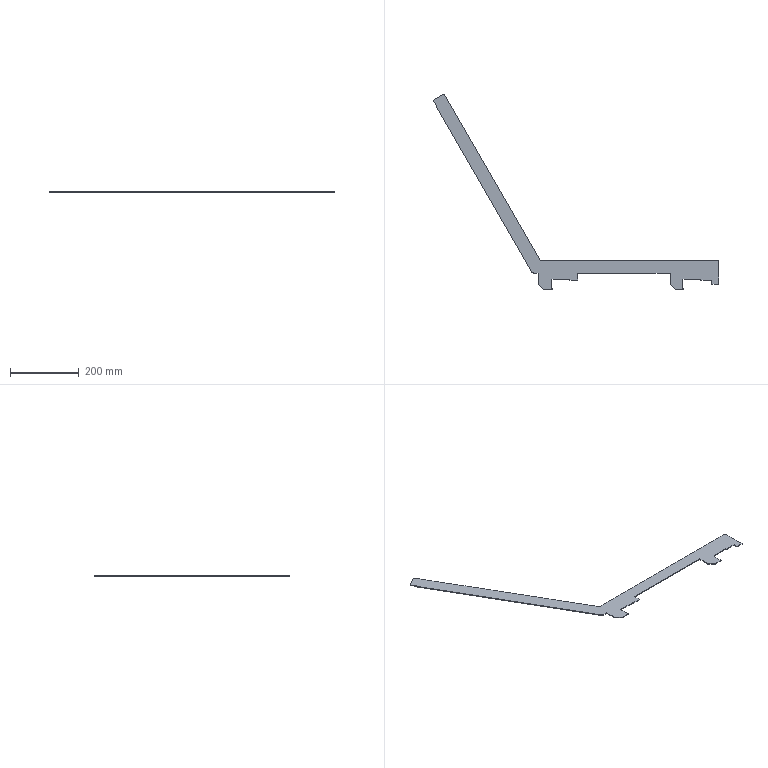Part | STEP file | zh001-1 | 1 solid | 35 faces | box 827.736 x 568.01 x 2 mm | volume 95326 mm3 | plane 32 | cylinder 3 | commonest cylinder face diameters 4 x2 20 x1
STEP:
#1=CARTESIAN_POINT('',(-259.956,-10.5,0.));
#2=VERTEX_POINT('',#1);
#3=CARTESIAN_POINT('',(-268.617,-5.5,0.));
#4=VERTEX_POINT('',#3);
#5=CARTESIAN_POINT('',(-259.956,-0.5,0.));
#6=DIRECTION('',(0.,0.,-1.));
#7=DIRECTION('',(1.,0.,0.));
#8=AXIS2_PLACEMENT_3D('',#5,#6,#7);
#9=CIRCLE('',#8,10.);
#10=EDGE_CURVE('',#2,#4,#9,.T.);
#11=ORIENTED_EDGE('',*,*,#10,.F.);
#12=CARTESIAN_POINT('',(-248.981,-10.5,0.));
#13=VERTEX_POINT('',#12);
#14=CARTESIAN_POINT('',(0.,-10.5,0.));
#15=DIRECTION('',(-1.,0.,0.));
#16=VECTOR('',#15,1000.);
#17=LINE('',#14,#16);
#18=EDGE_CURVE('',#13,#2,#17,.T.);
#19=ORIENTED_EDGE('',*,*,#18,.F.);
#20=CARTESIAN_POINT('',(-248.981,-43.,0.));
#21=VERTEX_POINT('',#20);
#22=CARTESIAN_POINT('',(-248.981,0.,0.));
#23=DIRECTION('',(0.,1.,0.));
#24=VECTOR('',#23,1000.);
#25=LINE('',#22,#24);
#26=EDGE_CURVE('',#21,#13,#25,.T.);
#27=ORIENTED_EDGE('',*,*,#26,.F.);
#28=CARTESIAN_POINT('',(-232.981,-59.,0.));
#29=VERTEX_POINT('',#28);
#30=CARTESIAN_POINT('',(-232.981,-59.,0.));
#31=DIRECTION('',(-0.7071,0.7071,0.));
#32=VECTOR('',#31,1000.);
#33=LINE('',#30,#32);
#34=EDGE_CURVE('',#29,#21,#33,.T.);
#35=ORIENTED_EDGE('',*,*,#34,.F.);
#36=CARTESIAN_POINT('',(-206.481,-59.,0.));
#37=VERTEX_POINT('',#36);
#38=CARTESIAN_POINT('',(0.,-59.,0.));
#39=DIRECTION('',(-1.,0.,0.));
#40=VECTOR('',#39,1000.);
#41=LINE('',#38,#40);
#42=EDGE_CURVE('',#37,#29,#41,.T.);
#43=ORIENTED_EDGE('',*,*,#42,.F.);
#44=CARTESIAN_POINT('',(-206.481,-56.,0.));
#45=VERTEX_POINT('',#44);
#46=CARTESIAN_POINT('',(-206.481,0.,0.));
#47=DIRECTION('',(0.,-1.,0.));
#48=VECTOR('',#47,1000.);
#49=LINE('',#46,#48);
#50=EDGE_CURVE('',#45,#37,#49,.T.);
#51=ORIENTED_EDGE('',*,*,#50,.F.);
#52=CARTESIAN_POINT('',(-208.981,-56.,0.));
#53=VERTEX_POINT('',#52);
#54=CARTESIAN_POINT('',(0.,-56.,0.));
#55=DIRECTION('',(1.,0.,0.));
#56=VECTOR('',#55,1000.);
#57=LINE('',#54,#56);
#58=EDGE_CURVE('',#53,#45,#57,.T.);
#59=ORIENTED_EDGE('',*,*,#58,.F.);
#60=CARTESIAN_POINT('',(-208.981,-28.,0.));
#61=VERTEX_POINT('',#60);
#62=CARTESIAN_POINT('',(-208.981,0.,0.));
#63=DIRECTION('',(0.,-1.,0.));
#64=VECTOR('',#63,1000.);
#65=LINE('',#62,#64);
#66=EDGE_CURVE('',#61,#53,#65,.T.);
#67=ORIENTED_EDGE('',*,*,#66,.F.);
#68=CARTESIAN_POINT('',(-156.981,-28.,0.));
#69=VERTEX_POINT('',#68);
#70=CARTESIAN_POINT('',(0.,-28.,0.));
#71=DIRECTION('',(-1.,0.,0.));
#72=VECTOR('',#71,1000.);
#73=LINE('',#70,#72);
#74=EDGE_CURVE('',#69,#61,#73,.T.);
#75=ORIENTED_EDGE('',*,*,#74,.F.);
#76=CARTESIAN_POINT('',(-156.981,-30.5,0.));
#77=VERTEX_POINT('',#76);
#78=CARTESIAN_POINT('',(-156.981,0.,0.));
#79=DIRECTION('',(0.,1.,0.));
#80=VECTOR('',#79,1000.);
#81=LINE('',#78,#80);
#82=EDGE_CURVE('',#77,#69,#81,.T.);
#83=ORIENTED_EDGE('',*,*,#82,.F.);
#84=CARTESIAN_POINT('',(-134.519,-30.5,0.));
#85=VERTEX_POINT('',#84);
#86=CARTESIAN_POINT('',(0.,-30.5,0.));
#87=DIRECTION('',(-1.,0.,0.));
#88=VECTOR('',#87,1000.);
#89=LINE('',#86,#88);
#90=EDGE_CURVE('',#85,#77,#89,.T.);
#91=ORIENTED_EDGE('',*,*,#90,.F.);
#92=CARTESIAN_POINT('',(-134.519,-10.5,0.));
#93=VERTEX_POINT('',#92);
#94=CARTESIAN_POINT('',(-134.519,0.,0.));
#95=DIRECTION('',(0.,-1.,0.));
#96=VECTOR('',#95,1000.);
#97=LINE('',#94,#96);
#98=EDGE_CURVE('',#93,#85,#97,.T.);
#99=ORIENTED_EDGE('',*,*,#98,.F.);
#100=CARTESIAN_POINT('',(133.519,-10.5,0.));
#101=VERTEX_POINT('',#100);
#102=CARTESIAN_POINT('',(0.,-10.5,0.));
#103=DIRECTION('',(-1.,0.,0.));
#104=VECTOR('',#103,1000.);
#105=LINE('',#102,#104);
#106=EDGE_CURVE('',#101,#93,#105,.T.);
#107=ORIENTED_EDGE('',*,*,#106,.F.);
#108=CARTESIAN_POINT('',(133.519,-43.,0.));
#109=VERTEX_POINT('',#108);
#110=CARTESIAN_POINT('',(133.519,0.,0.));
#111=DIRECTION('',(0.,1.,0.));
#112=VECTOR('',#111,1000.);
#113=LINE('',#110,#112);
#114=EDGE_CURVE('',#109,#101,#113,.T.);
#115=ORIENTED_EDGE('',*,*,#114,.F.);
#116=CARTESIAN_POINT('',(149.519,-59.,0.));
#117=VERTEX_POINT('',#116);
#118=CARTESIAN_POINT('',(149.519,-59.,0.));
#119=DIRECTION('',(-0.7071,0.7071,0.));
#120=VECTOR('',#119,1000.);
#121=LINE('',#118,#120);
#122=EDGE_CURVE('',#117,#109,#121,.T.);
#123=ORIENTED_EDGE('',*,*,#122,.F.);
#124=CARTESIAN_POINT('',(173.519,-59.,0.));
#125=VERTEX_POINT('',#124);
#126=CARTESIAN_POINT('',(0.,-59.,0.));
#127=DIRECTION('',(-1.,0.,0.));
#128=VECTOR('',#127,1000.);
#129=LINE('',#126,#128);
#130=EDGE_CURVE('',#125,#117,#129,.T.);
#131=ORIENTED_EDGE('',*,*,#130,.F.);
#132=CARTESIAN_POINT('',(173.519,-56.,0.));
#133=VERTEX_POINT('',#132);
#134=CARTESIAN_POINT('',(173.519,0.,0.));
#135=DIRECTION('',(0.,-1.,0.));
#136=VECTOR('',#135,1000.);
#137=LINE('',#134,#136);
#138=EDGE_CURVE('',#133,#125,#137,.T.);
#139=ORIENTED_EDGE('',*,*,#138,.F.);
#140=CARTESIAN_POINT('',(171.019,-56.,0.));
#141=VERTEX_POINT('',#140);
#142=CARTESIAN_POINT('',(0.,-56.,0.));
#143=DIRECTION('',(1.,0.,0.));
#144=VECTOR('',#143,1000.);
#145=LINE('',#142,#144);
#146=EDGE_CURVE('',#141,#133,#145,.T.);
#147=ORIENTED_EDGE('',*,*,#146,.F.);
#148=CARTESIAN_POINT('',(171.019,-28.,0.));
#149=VERTEX_POINT('',#148);
#150=CARTESIAN_POINT('',(171.019,0.,0.));
#151=DIRECTION('',(0.,-1.,0.));
#152=VECTOR('',#151,1000.);
#153=LINE('',#150,#152);
#154=EDGE_CURVE('',#149,#141,#153,.T.);
#155=ORIENTED_EDGE('',*,*,#154,.F.);
#156=CARTESIAN_POINT('',(223.019,-28.,0.));
#157=VERTEX_POINT('',#156);
#158=CARTESIAN_POINT('',(0.,-28.,0.));
#159=DIRECTION('',(-1.,0.,0.));
#160=VECTOR('',#159,1000.);
#161=LINE('',#158,#160);
#162=EDGE_CURVE('',#157,#149,#161,.T.);
#163=ORIENTED_EDGE('',*,*,#162,.F.);
#164=CARTESIAN_POINT('',(223.019,-30.5,0.));
#165=VERTEX_POINT('',#164);
#166=CARTESIAN_POINT('',(223.019,0.,0.));
#167=DIRECTION('',(0.,1.,0.));
#168=VECTOR('',#167,1000.);
#169=LINE('',#166,#168);
#170=EDGE_CURVE('',#165,#157,#169,.T.);
#171=ORIENTED_EDGE('',*,*,#170,.F.);
#172=CARTESIAN_POINT('',(254.235,-30.5,0.));
#173=VERTEX_POINT('',#172);
#174=CARTESIAN_POINT('',(0.,-30.5,0.));
#175=DIRECTION('',(-1.,0.,0.));
#176=VECTOR('',#175,1000.);
#177=LINE('',#174,#176);
#178=EDGE_CURVE('',#173,#165,#177,.T.);
#179=ORIENTED_EDGE('',*,*,#178,.F.);
#180=CARTESIAN_POINT('',(254.235,-42.5,0.));
#181=VERTEX_POINT('',#180);
#182=CARTESIAN_POINT('',(254.235,0.,0.));
#183=DIRECTION('',(0.,1.,0.));
#184=VECTOR('',#183,1000.);
#185=LINE('',#182,#184);
#186=EDGE_CURVE('',#181,#173,#185,.T.);
#187=ORIENTED_EDGE('',*,*,#186,.F.);
#188=CARTESIAN_POINT('',(274.519,-42.5,0.));
#189=VERTEX_POINT('',#188);
#190=CARTESIAN_POINT('',(0.,-42.5,0.));
#191=DIRECTION('',(-1.,0.,0.));
#192=VECTOR('',#191,1000.);
#193=LINE('',#190,#192);
#194=EDGE_CURVE('',#189,#181,#193,.T.);
#195=ORIENTED_EDGE('',*,*,#194,.F.);
#196=CARTESIAN_POINT('',(274.519,23.5,0.));
#197=VERTEX_POINT('',#196);
#198=CARTESIAN_POINT('',(274.519,0.,0.));
#199=DIRECTION('',(0.,-1.,0.));
#200=VECTOR('',#199,1000.);
#201=LINE('',#198,#200);
#202=EDGE_CURVE('',#197,#189,#201,.T.);
#203=ORIENTED_EDGE('',*,*,#202,.F.);
#204=CARTESIAN_POINT('',(272.519,25.5,0.));
#205=VERTEX_POINT('',#204);
#206=CARTESIAN_POINT('',(272.519,23.5,0.));
#207=DIRECTION('',(0.,0.,-1.));
#208=DIRECTION('',(1.,0.,0.));
#209=AXIS2_PLACEMENT_3D('',#206,#207,#208);
#210=CIRCLE('',#209,2.);
#211=EDGE_CURVE('',#205,#197,#210,.T.);
#212=ORIENTED_EDGE('',*,*,#211,.F.);
#213=CARTESIAN_POINT('',(-242.636,25.5,0.));
#214=VERTEX_POINT('',#213);
#215=CARTESIAN_POINT('',(0.,25.5,0.));
#216=DIRECTION('',(1.,0.,0.));
#217=VECTOR('',#216,1000.);
#218=LINE('',#215,#217);
#219=EDGE_CURVE('',#214,#205,#218,.T.);
#220=ORIENTED_EDGE('',*,*,#219,.F.);
#221=CARTESIAN_POINT('',(-521.213,508.01,0.));
#222=VERTEX_POINT('',#221);
#223=CARTESIAN_POINT('',(-521.213,508.01,0.));
#224=DIRECTION('',(0.5,-0.866,0.));
#225=VECTOR('',#224,1000.);
#226=LINE('',#223,#225);
#227=EDGE_CURVE('',#222,#214,#226,.T.);
#228=ORIENTED_EDGE('',*,*,#227,.F.);
#229=CARTESIAN_POINT('',(-523.945,508.742,0.));
#230=VERTEX_POINT('',#229);
#231=CARTESIAN_POINT('',(-522.945,507.01,0.));
#232=DIRECTION('',(0.,0.,-1.));
#233=DIRECTION('',(1.,0.,0.));
#234=AXIS2_PLACEMENT_3D('',#231,#232,#233);
#235=CIRCLE('',#234,2.);
#236=EDGE_CURVE('',#230,#222,#235,.T.);
#237=ORIENTED_EDGE('',*,*,#236,.F.);
#238=CARTESIAN_POINT('',(-553.217,491.842,0.));
#239=VERTEX_POINT('',#238);
#240=CARTESIAN_POINT('',(-553.217,491.842,0.));
#241=DIRECTION('',(0.866,0.5,0.));
#242=VECTOR('',#241,1000.);
#243=LINE('',#240,#242);
#244=EDGE_CURVE('',#239,#230,#243,.T.);
#245=ORIENTED_EDGE('',*,*,#244,.F.);
#246=CARTESIAN_POINT('',(-543.117,474.348,0.));
#247=VERTEX_POINT('',#246);
#248=CARTESIAN_POINT('',(-543.117,474.348,0.));
#249=DIRECTION('',(-0.5,0.866,0.));
#250=VECTOR('',#249,1000.);
#251=LINE('',#248,#250);
#252=EDGE_CURVE('',#247,#239,#251,.T.);
#253=ORIENTED_EDGE('',*,*,#252,.F.);
#254=CARTESIAN_POINT('',(-545.022,473.248,0.));
#255=VERTEX_POINT('',#254);
#256=CARTESIAN_POINT('',(-545.022,473.248,0.));
#257=DIRECTION('',(0.866,0.5,0.));
#258=VECTOR('',#257,1000.);
#259=LINE('',#256,#258);
#260=EDGE_CURVE('',#255,#247,#259,.T.);
#261=ORIENTED_EDGE('',*,*,#260,.F.);
#262=CARTESIAN_POINT('',(-268.617,-5.5,0.));
#263=DIRECTION('',(-0.5,0.866,0.));
#264=VECTOR('',#263,1000.);
#265=LINE('',#262,#264);
#266=EDGE_CURVE('',#4,#255,#265,.T.);
#267=ORIENTED_EDGE('',*,*,#266,.F.);
#268=EDGE_LOOP('',(#11,#19,#27,#35,#43,#51,#59,#67,#75,#83,#91,#99,#107,#115,#123,#131,#139,#147,#155,#163,#171,#179,#187,#195,#203,#212,#220,#228,#237,#245,#253,#261,#267));
#269=FACE_OUTER_BOUND('',#268,.T.);
#270=CARTESIAN_POINT('',(0.,0.,0.));
#271=DIRECTION('',(0.,0.,-1.));
#272=DIRECTION('',(-1.,0.,0.));
#273=AXIS2_PLACEMENT_3D('',#270,#271,#272);
#274=PLANE('',#273);
#275=ADVANCED_FACE('',(#269),#274,.F.);
#276=ORIENTED_EDGE('',*,*,#266,.T.);
#277=CARTESIAN_POINT('',(-545.022,473.248,-2.));
#278=VERTEX_POINT('',#277);
#279=CARTESIAN_POINT('',(-545.022,473.248,-2.));
#280=DIRECTION('',(0.,0.,-1.));
#281=VECTOR('',#280,1000.);
#282=LINE('',#279,#281);
#283=EDGE_CURVE('',#255,#278,#282,.T.);
#284=ORIENTED_EDGE('',*,*,#283,.T.);
#285=CARTESIAN_POINT('',(-268.617,-5.5,-2.));
#286=VERTEX_POINT('',#285);
#287=CARTESIAN_POINT('',(-545.022,473.248,-2.));
#288=DIRECTION('',(0.5,-0.866,0.));
#289=VECTOR('',#288,1000.);
#290=LINE('',#287,#289);
#291=EDGE_CURVE('',#278,#286,#290,.T.);
#292=ORIENTED_EDGE('',*,*,#291,.T.);
#293=CARTESIAN_POINT('',(-268.617,-5.5,-2.));
#294=DIRECTION('',(0.,0.,1.));
#295=VECTOR('',#294,1000.);
#296=LINE('',#293,#295);
#297=EDGE_CURVE('',#286,#4,#296,.T.);
#298=ORIENTED_EDGE('',*,*,#297,.T.);
#299=EDGE_LOOP('',(#276,#284,#292,#298));
#300=FACE_OUTER_BOUND('',#299,.T.);
#301=CARTESIAN_POINT('',(-545.022,473.248,-2.));
#302=DIRECTION('',(-0.866,-0.5,0.));
#303=DIRECTION('',(0.5,-0.866,0.));
#304=AXIS2_PLACEMENT_3D('',#301,#302,#303);
#305=PLANE('',#304);
#306=ADVANCED_FACE('',(#300),#305,.T.);
#307=ORIENTED_EDGE('',*,*,#10,.T.);
#308=ORIENTED_EDGE('',*,*,#297,.F.);
#309=CARTESIAN_POINT('',(-259.956,-10.5,-2.));
#310=VERTEX_POINT('',#309);
#311=CARTESIAN_POINT('',(-259.956,-0.5,-2.));
#312=DIRECTION('',(0.,0.,1.));
#313=DIRECTION('',(1.,0.,0.));
#314=AXIS2_PLACEMENT_3D('',#311,#312,#313);
#315=CIRCLE('',#314,10.);
#316=EDGE_CURVE('',#286,#310,#315,.T.);
#317=ORIENTED_EDGE('',*,*,#316,.T.);
#318=CARTESIAN_POINT('',(-259.956,-10.5,-2.));
#319=DIRECTION('',(0.,0.,1.));
#320=VECTOR('',#319,1000.);
#321=LINE('',#318,#320);
#322=EDGE_CURVE('',#310,#2,#321,.T.);
#323=ORIENTED_EDGE('',*,*,#322,.T.);
#324=EDGE_LOOP('',(#307,#308,#317,#323));
#325=FACE_OUTER_BOUND('',#324,.T.);
#326=CARTESIAN_POINT('',(-259.956,-0.5,-2.));
#327=DIRECTION('',(0.,0.,1.));
#328=DIRECTION('',(1.,0.,0.));
#329=AXIS2_PLACEMENT_3D('',#326,#327,#328);
#330=CYLINDRICAL_SURFACE('',#329,10.);
#331=ADVANCED_FACE('',(#325),#330,.T.);
#332=CARTESIAN_POINT('',(-248.981,-10.5,-2.));
#333=VERTEX_POINT('',#332);
#334=CARTESIAN_POINT('',(-248.981,-10.5,-2.));
#335=DIRECTION('',(1.,0.,0.));
#336=VECTOR('',#335,1000.);
#337=LINE('',#334,#336);
#338=EDGE_CURVE('',#310,#333,#337,.T.);
#339=ORIENTED_EDGE('',*,*,#338,.T.);
#340=CARTESIAN_POINT('',(-248.981,-10.5,-2.));
#341=DIRECTION('',(0.,0.,1.));
#342=VECTOR('',#341,1000.);
#343=LINE('',#340,#342);
#344=EDGE_CURVE('',#333,#13,#343,.T.);
#345=ORIENTED_EDGE('',*,*,#344,.T.);
#346=ORIENTED_EDGE('',*,*,#18,.T.);
#347=ORIENTED_EDGE('',*,*,#322,.F.);
#348=EDGE_LOOP('',(#339,#345,#346,#347));
#349=FACE_OUTER_BOUND('',#348,.T.);
#350=CARTESIAN_POINT('',(-248.981,-10.5,-2.));
#351=DIRECTION('',(0.,-1.,0.));
#352=DIRECTION('',(1.,0.,0.));
#353=AXIS2_PLACEMENT_3D('',#350,#351,#352);
#354=PLANE('',#353);
#355=ADVANCED_FACE('',(#349),#354,.T.);
#356=ORIENTED_EDGE('',*,*,#26,.T.);
#357=ORIENTED_EDGE('',*,*,#344,.F.);
#358=CARTESIAN_POINT('',(-248.981,-43.,-2.));
#359=VERTEX_POINT('',#358);
#360=CARTESIAN_POINT('',(-248.981,-59.,-2.));
#361=DIRECTION('',(0.,-1.,0.));
#362=VECTOR('',#361,1000.);
#363=LINE('',#360,#362);
#364=EDGE_CURVE('',#333,#359,#363,.T.);
#365=ORIENTED_EDGE('',*,*,#364,.T.);
#366=CARTESIAN_POINT('',(-248.981,-43.,-2.));
#367=DIRECTION('',(0.,0.,1.));
#368=VECTOR('',#367,1000.);
#369=LINE('',#366,#368);
#370=EDGE_CURVE('',#359,#21,#369,.T.);
#371=ORIENTED_EDGE('',*,*,#370,.T.);
#372=EDGE_LOOP('',(#356,#357,#365,#371));
#373=FACE_OUTER_BOUND('',#372,.T.);
#374=CARTESIAN_POINT('',(-248.981,-59.,-2.));
#375=DIRECTION('',(-1.,0.,0.));
#376=DIRECTION('',(0.,-1.,0.));
#377=AXIS2_PLACEMENT_3D('',#374,#375,#376);
#378=PLANE('',#377);
#379=ADVANCED_FACE('',(#373),#378,.T.);
#380=CARTESIAN_POINT('',(-232.981,-59.,-2.));
#381=VERTEX_POINT('',#380);
#382=CARTESIAN_POINT('',(-232.981,-59.,-2.));
#383=DIRECTION('',(0.,0.,-1.));
#384=VECTOR('',#383,1000.);
#385=LINE('',#382,#384);
#386=EDGE_CURVE('',#29,#381,#385,.T.);
#387=ORIENTED_EDGE('',*,*,#386,.F.);
#388=ORIENTED_EDGE('',*,*,#34,.T.);
#389=ORIENTED_EDGE('',*,*,#370,.F.);
#390=CARTESIAN_POINT('',(-248.981,-43.,-2.));
#391=DIRECTION('',(-0.7071,0.7071,0.));
#392=VECTOR('',#391,1000.);
#393=LINE('',#390,#392);
#394=EDGE_CURVE('',#381,#359,#393,.T.);
#395=ORIENTED_EDGE('',*,*,#394,.F.);
#396=EDGE_LOOP('',(#387,#388,#389,#395));
#397=FACE_OUTER_BOUND('',#396,.T.);
#398=CARTESIAN_POINT('',(-248.981,-43.,-2.));
#399=DIRECTION('',(0.7071,0.7071,0.));
#400=DIRECTION('',(-0.7071,0.7071,0.));
#401=AXIS2_PLACEMENT_3D('',#398,#399,#400);
#402=PLANE('',#401);
#403=ADVANCED_FACE('',(#397),#402,.F.);
#404=CARTESIAN_POINT('',(-206.481,-59.,-2.));
#405=VERTEX_POINT('',#404);
#406=CARTESIAN_POINT('',(-206.481,-59.,-2.));
#407=DIRECTION('',(1.,0.,0.));
#408=VECTOR('',#407,1000.);
#409=LINE('',#406,#408);
#410=EDGE_CURVE('',#381,#405,#409,.T.);
#411=ORIENTED_EDGE('',*,*,#410,.T.);
#412=CARTESIAN_POINT('',(-206.481,-59.,-2.));
#413=DIRECTION('',(0.,0.,1.));
#414=VECTOR('',#413,1000.);
#415=LINE('',#412,#414);
#416=EDGE_CURVE('',#405,#37,#415,.T.);
#417=ORIENTED_EDGE('',*,*,#416,.T.);
#418=ORIENTED_EDGE('',*,*,#42,.T.);
#419=ORIENTED_EDGE('',*,*,#386,.T.);
#420=EDGE_LOOP('',(#411,#417,#418,#419));
#421=FACE_OUTER_BOUND('',#420,.T.);
#422=CARTESIAN_POINT('',(-206.481,-59.,-2.));
#423=DIRECTION('',(0.,-1.,0.));
#424=DIRECTION('',(1.,0.,0.));
#425=AXIS2_PLACEMENT_3D('',#422,#423,#424);
#426=PLANE('',#425);
#427=ADVANCED_FACE('',(#421),#426,.T.);
#428=CARTESIAN_POINT('',(-206.481,-56.,-2.));
#429=VERTEX_POINT('',#428);
#430=CARTESIAN_POINT('',(-206.481,-56.,-2.));
#431=DIRECTION('',(0.,1.,0.));
#432=VECTOR('',#431,1000.);
#433=LINE('',#430,#432);
#434=EDGE_CURVE('',#405,#429,#433,.T.);
#435=ORIENTED_EDGE('',*,*,#434,.T.);
#436=CARTESIAN_POINT('',(-206.481,-56.,-2.));
#437=DIRECTION('',(0.,0.,1.));
#438=VECTOR('',#437,1000.);
#439=LINE('',#436,#438);
#440=EDGE_CURVE('',#429,#45,#439,.T.);
#441=ORIENTED_EDGE('',*,*,#440,.T.);
#442=ORIENTED_EDGE('',*,*,#50,.T.);
#443=ORIENTED_EDGE('',*,*,#416,.F.);
#444=EDGE_LOOP('',(#435,#441,#442,#443));
#445=FACE_OUTER_BOUND('',#444,.T.);
#446=CARTESIAN_POINT('',(-206.481,-56.,-2.));
#447=DIRECTION('',(1.,0.,0.));
#448=DIRECTION('',(0.,1.,0.));
#449=AXIS2_PLACEMENT_3D('',#446,#447,#448);
#450=PLANE('',#449);
#451=ADVANCED_FACE('',(#445),#450,.T.);
#452=CARTESIAN_POINT('',(-208.981,-56.,-2.));
#453=VERTEX_POINT('',#452);
#454=CARTESIAN_POINT('',(-208.981,-56.,-2.));
#455=DIRECTION('',(-1.,0.,0.));
#456=VECTOR('',#455,1000.);
#457=LINE('',#454,#456);
#458=EDGE_CURVE('',#429,#453,#457,.T.);
#459=ORIENTED_EDGE('',*,*,#458,.T.);
#460=CARTESIAN_POINT('',(-208.981,-56.,-2.));
#461=DIRECTION('',(0.,0.,1.));
#462=VECTOR('',#461,1000.);
#463=LINE('',#460,#462);
#464=EDGE_CURVE('',#453,#53,#463,.T.);
#465=ORIENTED_EDGE('',*,*,#464,.T.);
#466=ORIENTED_EDGE('',*,*,#58,.T.);
#467=ORIENTED_EDGE('',*,*,#440,.F.);
#468=EDGE_LOOP('',(#459,#465,#466,#467));
#469=FACE_OUTER_BOUND('',#468,.T.);
#470=CARTESIAN_POINT('',(-208.981,-56.,-2.));
#471=DIRECTION('',(0.,1.,0.));
#472=DIRECTION('',(-1.,0.,0.));
#473=AXIS2_PLACEMENT_3D('',#470,#471,#472);
#474=PLANE('',#473);
#475=ADVANCED_FACE('',(#469),#474,.T.);
#476=CARTESIAN_POINT('',(-208.981,-28.,-2.));
#477=VERTEX_POINT('',#476);
#478=CARTESIAN_POINT('',(-208.981,-56.,-2.));
#479=DIRECTION('',(0.,1.,0.));
#480=VECTOR('',#479,1000.);
#481=LINE('',#478,#480);
#482=EDGE_CURVE('',#453,#477,#481,.T.);
#483=ORIENTED_EDGE('',*,*,#482,.T.);
#484=CARTESIAN_POINT('',(-208.981,-28.,-2.));
#485=DIRECTION('',(0.,0.,1.));
#486=VECTOR('',#485,1000.);
#487=LINE('',#484,#486);
#488=EDGE_CURVE('',#477,#61,#487,.T.);
#489=ORIENTED_EDGE('',*,*,#488,.T.);
#490=ORIENTED_EDGE('',*,*,#66,.T.);
#491=ORIENTED_EDGE('',*,*,#464,.F.);
#492=EDGE_LOOP('',(#483,#489,#490,#491));
#493=FACE_OUTER_BOUND('',#492,.T.);
#494=CARTESIAN_POINT('',(-208.981,-56.,-2.));
#495=DIRECTION('',(1.,0.,0.));
#496=DIRECTION('',(0.,1.,0.));
#497=AXIS2_PLACEMENT_3D('',#494,#495,#496);
#498=PLANE('',#497);
#499=ADVANCED_FACE('',(#493),#498,.T.);
#500=CARTESIAN_POINT('',(-156.981,-28.,-2.));
#501=VERTEX_POINT('',#500);
#502=CARTESIAN_POINT('',(-208.981,-28.,-2.));
#503=DIRECTION('',(1.,0.,0.));
#504=VECTOR('',#503,1000.);
#505=LINE('',#502,#504);
#506=EDGE_CURVE('',#477,#501,#505,.T.);
#507=ORIENTED_EDGE('',*,*,#506,.T.);
#508=CARTESIAN_POINT('',(-156.981,-28.,-2.));
#509=DIRECTION('',(0.,0.,1.));
#510=VECTOR('',#509,1000.);
#511=LINE('',#508,#510);
#512=EDGE_CURVE('',#501,#69,#511,.T.);
#513=ORIENTED_EDGE('',*,*,#512,.T.);
#514=ORIENTED_EDGE('',*,*,#74,.T.);
#515=ORIENTED_EDGE('',*,*,#488,.F.);
#516=EDGE_LOOP('',(#507,#513,#514,#515));
#517=FACE_OUTER_BOUND('',#516,.T.);
#518=CARTESIAN_POINT('',(-208.981,-28.,-2.));
#519=DIRECTION('',(0.,-1.,0.));
#520=DIRECTION('',(1.,0.,0.));
#521=AXIS2_PLACEMENT_3D('',#518,#519,#520);
#522=PLANE('',#521);
#523=ADVANCED_FACE('',(#517),#522,.T.);
#524=CARTESIAN_POINT('',(-156.981,-30.5,-2.));
#525=VERTEX_POINT('',#524);
#526=CARTESIAN_POINT('',(-156.981,-28.,-2.));
#527=DIRECTION('',(0.,-1.,0.));
#528=VECTOR('',#527,1000.);
#529=LINE('',#526,#528);
#530=EDGE_CURVE('',#501,#525,#529,.T.);
#531=ORIENTED_EDGE('',*,*,#530,.T.);
#532=CARTESIAN_POINT('',(-156.981,-30.5,-2.));
#533=DIRECTION('',(0.,0.,1.));
#534=VECTOR('',#533,1000.);
#535=LINE('',#532,#534);
#536=EDGE_CURVE('',#525,#77,#535,.T.);
#537=ORIENTED_EDGE('',*,*,#536,.T.);
#538=ORIENTED_EDGE('',*,*,#82,.T.);
#539=ORIENTED_EDGE('',*,*,#512,.F.);
#540=EDGE_LOOP('',(#531,#537,#538,#539));
#541=FACE_OUTER_BOUND('',#540,.T.);
#542=CARTESIAN_POINT('',(-156.981,-28.,-2.));
#543=DIRECTION('',(-1.,0.,0.));
#544=DIRECTION('',(0.,0.,1.));
#545=AXIS2_PLACEMENT_3D('',#542,#543,#544);
#546=PLANE('',#545);
#547=ADVANCED_FACE('',(#541),#546,.T.);
#548=CARTESIAN_POINT('',(-134.519,-30.5,-2.));
#549=VERTEX_POINT('',#548);
#550=CARTESIAN_POINT('',(-156.981,-30.5,-2.));
#551=DIRECTION('',(1.,0.,0.));
#552=VECTOR('',#551,1000.);
#553=LINE('',#550,#552);
#554=EDGE_CURVE('',#525,#549,#553,.T.);
#555=ORIENTED_EDGE('',*,*,#554,.T.);
#556=CARTESIAN_POINT('',(-134.519,-30.5,-2.));
#557=DIRECTION('',(0.,0.,1.));
#558=VECTOR('',#557,1000.);
#559=LINE('',#556,#558);
#560=EDGE_CURVE('',#549,#85,#559,.T.);
#561=ORIENTED_EDGE('',*,*,#560,.T.);
#562=ORIENTED_EDGE('',*,*,#90,.T.);
#563=ORIENTED_EDGE('',*,*,#536,.F.);
#564=EDGE_LOOP('',(#555,#561,#562,#563));
#565=FACE_OUTER_BOUND('',#564,.T.);
#566=CARTESIAN_POINT('',(-156.981,-30.5,-2.));
#567=DIRECTION('',(0.,-1.,0.));
#568=DIRECTION('',(1.,0.,0.));
#569=AXIS2_PLACEMENT_3D('',#566,#567,#568);
#570=PLANE('',#569);
#571=ADVANCED_FACE('',(#565),#570,.T.);
#572=CARTESIAN_POINT('',(-134.519,-10.5,-2.));
#573=VERTEX_POINT('',#572);
#574=CARTESIAN_POINT('',(-134.519,-30.5,-2.));
#575=DIRECTION('',(0.,1.,0.));
#576=VECTOR('',#575,1000.);
#577=LINE('',#574,#576);
#578=EDGE_CURVE('',#549,#573,#577,.T.);
#579=ORIENTED_EDGE('',*,*,#578,.T.);
#580=CARTESIAN_POINT('',(-134.519,-10.5,-2.));
#581=DIRECTION('',(0.,0.,1.));
#582=VECTOR('',#581,1000.);
#583=LINE('',#580,#582);
#584=EDGE_CURVE('',#573,#93,#583,.T.);
#585=ORIENTED_EDGE('',*,*,#584,.T.);
#586=ORIENTED_EDGE('',*,*,#98,.T.);
#587=ORIENTED_EDGE('',*,*,#560,.F.);
#588=EDGE_LOOP('',(#579,#585,#586,#587));
#589=FACE_OUTER_BOUND('',#588,.T.);
#590=CARTESIAN_POINT('',(-134.519,-30.5,-2.));
#591=DIRECTION('',(1.,0.,0.));
#592=DIRECTION('',(0.,1.,0.));
#593=AXIS2_PLACEMENT_3D('',#590,#591,#592);
#594=PLANE('',#593);
#595=ADVANCED_FACE('',(#589),#594,.T.);
#596=CARTESIAN_POINT('',(133.519,-10.5,-2.));
#597=VERTEX_POINT('',#596);
#598=CARTESIAN_POINT('',(-134.519,-10.5,-2.));
#599=DIRECTION('',(1.,0.,0.));
#600=VECTOR('',#599,1000.);
#601=LINE('',#598,#600);
#602=EDGE_CURVE('',#573,#597,#601,.T.);
#603=ORIENTED_EDGE('',*,*,#602,.T.);
#604=CARTESIAN_POINT('',(133.519,-10.5,-2.));
#605=DIRECTION('',(0.,0.,1.));
#606=VECTOR('',#605,1000.);
#607=LINE('',#604,#606);
#608=EDGE_CURVE('',#597,#101,#607,.T.);
#609=ORIENTED_EDGE('',*,*,#608,.T.);
#610=ORIENTED_EDGE('',*,*,#106,.T.);
#611=ORIENTED_EDGE('',*,*,#584,.F.);
#612=EDGE_LOOP('',(#603,#609,#610,#611));
#613=FACE_OUTER_BOUND('',#612,.T.);
#614=CARTESIAN_POINT('',(-134.519,-10.5,-2.));
#615=DIRECTION('',(0.,-1.,0.));
#616=DIRECTION('',(1.,0.,0.));
#617=AXIS2_PLACEMENT_3D('',#614,#615,#616);
#618=PLANE('',#617);
#619=ADVANCED_FACE('',(#613),#618,.T.);
#620=ORIENTED_EDGE('',*,*,#114,.T.);
#621=ORIENTED_EDGE('',*,*,#608,.F.);
#622=CARTESIAN_POINT('',(133.519,-43.,-2.));
#623=VERTEX_POINT('',#622);
#624=CARTESIAN_POINT('',(133.519,-10.5,-2.));
#625=DIRECTION('',(0.,-1.,0.));
#626=VECTOR('',#625,1000.);
#627=LINE('',#624,#626);
#628=EDGE_CURVE('',#597,#623,#627,.T.);
#629=ORIENTED_EDGE('',*,*,#628,.T.);
#630=CARTESIAN_POINT('',(133.519,-43.,-2.));
#631=DIRECTION('',(0.,0.,1.));
#632=VECTOR('',#631,1000.);
#633=LINE('',#630,#632);
#634=EDGE_CURVE('',#623,#109,#633,.T.);
#635=ORIENTED_EDGE('',*,*,#634,.T.);
#636=EDGE_LOOP('',(#620,#621,#629,#635));
#637=FACE_OUTER_BOUND('',#636,.T.);
#638=CARTESIAN_POINT('',(133.519,-10.5,-2.));
#639=DIRECTION('',(-1.,0.,0.));
#640=DIRECTION('',(0.,-1.,0.));
#641=AXIS2_PLACEMENT_3D('',#638,#639,#640);
#642=PLANE('',#641);
#643=ADVANCED_FACE('',(#637),#642,.T.);
#644=CARTESIAN_POINT('',(149.519,-59.,-2.));
#645=VERTEX_POINT('',#644);
#646=CARTESIAN_POINT('',(149.519,-59.,-2.));
#647=DIRECTION('',(0.,0.,-1.));
#648=VECTOR('',#647,1000.);
#649=LINE('',#646,#648);
#650=EDGE_CURVE('',#117,#645,#649,.T.);
#651=ORIENTED_EDGE('',*,*,#650,.F.);
#652=ORIENTED_EDGE('',*,*,#122,.T.);
#653=ORIENTED_EDGE('',*,*,#634,.F.);
#654=CARTESIAN_POINT('',(133.519,-43.,-2.));
#655=DIRECTION('',(-0.7071,0.7071,0.));
#656=VECTOR('',#655,1000.);
#657=LINE('',#654,#656);
#658=EDGE_CURVE('',#645,#623,#657,.T.);
#659=ORIENTED_EDGE('',*,*,#658,.F.);
#660=EDGE_LOOP('',(#651,#652,#653,#659));
#661=FACE_OUTER_BOUND('',#660,.T.);
#662=CARTESIAN_POINT('',(133.519,-43.,-2.));
#663=DIRECTION('',(0.7071,0.7071,0.));
#664=DIRECTION('',(-0.7071,0.7071,0.));
#665=AXIS2_PLACEMENT_3D('',#662,#663,#664);
#666=PLANE('',#665);
#667=ADVANCED_FACE('',(#661),#666,.F.);
#668=CARTESIAN_POINT('',(173.519,-59.,-2.));
#669=VERTEX_POINT('',#668);
#670=CARTESIAN_POINT('',(133.519,-59.,-2.));
#671=DIRECTION('',(1.,0.,0.));
#672=VECTOR('',#671,1000.);
#673=LINE('',#670,#672);
#674=EDGE_CURVE('',#645,#669,#673,.T.);
#675=ORIENTED_EDGE('',*,*,#674,.T.);
#676=CARTESIAN_POINT('',(173.519,-59.,-2.));
#677=DIRECTION('',(0.,0.,1.));
#678=VECTOR('',#677,1000.);
#679=LINE('',#676,#678);
#680=EDGE_CURVE('',#669,#125,#679,.T.);
#681=ORIENTED_EDGE('',*,*,#680,.T.);
#682=ORIENTED_EDGE('',*,*,#130,.T.);
#683=ORIENTED_EDGE('',*,*,#650,.T.);
#684=EDGE_LOOP('',(#675,#681,#682,#683));
#685=FACE_OUTER_BOUND('',#684,.T.);
#686=CARTESIAN_POINT('',(133.519,-59.,-2.));
#687=DIRECTION('',(0.,-1.,0.));
#688=DIRECTION('',(1.,0.,0.));
#689=AXIS2_PLACEMENT_3D('',#686,#687,#688);
#690=PLANE('',#689);
#691=ADVANCED_FACE('',(#685),#690,.T.);
#692=CARTESIAN_POINT('',(173.519,-56.,-2.));
#693=VERTEX_POINT('',#692);
#694=CARTESIAN_POINT('',(173.519,-56.,-2.));
#695=DIRECTION('',(0.,1.,0.));
#696=VECTOR('',#695,1000.);
#697=LINE('',#694,#696);
#698=EDGE_CURVE('',#669,#693,#697,.T.);
#699=ORIENTED_EDGE('',*,*,#698,.T.);
#700=CARTESIAN_POINT('',(173.519,-56.,-2.));
#701=DIRECTION('',(0.,0.,1.));
#702=VECTOR('',#701,1000.);
#703=LINE('',#700,#702);
#704=EDGE_CURVE('',#693,#133,#703,.T.);
#705=ORIENTED_EDGE('',*,*,#704,.T.);
#706=ORIENTED_EDGE('',*,*,#138,.T.);
#707=ORIENTED_EDGE('',*,*,#680,.F.);
#708=EDGE_LOOP('',(#699,#705,#706,#707));
#709=FACE_OUTER_BOUND('',#708,.T.);
#710=CARTESIAN_POINT('',(173.519,-56.,-2.));
#711=DIRECTION('',(1.,0.,0.));
#712=DIRECTION('',(0.,1.,0.));
#713=AXIS2_PLACEMENT_3D('',#710,#711,#712);
#714=PLANE('',#713);
#715=ADVANCED_FACE('',(#709),#714,.T.);
#716=CARTESIAN_POINT('',(171.019,-56.,-2.));
#717=VERTEX_POINT('',#716);
#718=CARTESIAN_POINT('',(171.019,-56.,-2.));
#719=DIRECTION('',(-1.,0.,0.));
#720=VECTOR('',#719,1000.);
#721=LINE('',#718,#720);
#722=EDGE_CURVE('',#693,#717,#721,.T.);
#723=ORIENTED_EDGE('',*,*,#722,.T.);
#724=CARTESIAN_POINT('',(171.019,-56.,-2.));
#725=DIRECTION('',(0.,0.,1.));
#726=VECTOR('',#725,1000.);
#727=LINE('',#724,#726);
#728=EDGE_CURVE('',#717,#141,#727,.T.);
#729=ORIENTED_EDGE('',*,*,#728,.T.);
#730=ORIENTED_EDGE('',*,*,#146,.T.);
#731=ORIENTED_EDGE('',*,*,#704,.F.);
#732=EDGE_LOOP('',(#723,#729,#730,#731));
#733=FACE_OUTER_BOUND('',#732,.T.);
#734=CARTESIAN_POINT('',(171.019,-56.,-2.));
#735=DIRECTION('',(0.,1.,0.));
#736=DIRECTION('',(-1.,0.,0.));
#737=AXIS2_PLACEMENT_3D('',#734,#735,#736);
#738=PLANE('',#737);
#739=ADVANCED_FACE('',(#733),#738,.T.);
#740=CARTESIAN_POINT('',(171.019,-28.,-2.));
#741=VERTEX_POINT('',#740);
#742=CARTESIAN_POINT('',(171.019,-56.,-2.));
#743=DIRECTION('',(0.,1.,0.));
#744=VECTOR('',#743,1000.);
#745=LINE('',#742,#744);
#746=EDGE_CURVE('',#717,#741,#745,.T.);
#747=ORIENTED_EDGE('',*,*,#746,.T.);
#748=CARTESIAN_POINT('',(171.019,-28.,-2.));
#749=DIRECTION('',(0.,0.,1.));
#750=VECTOR('',#749,1000.);
#751=LINE('',#748,#750);
#752=EDGE_CURVE('',#741,#149,#751,.T.);
#753=ORIENTED_EDGE('',*,*,#752,.T.);
#754=ORIENTED_EDGE('',*,*,#154,.T.);
#755=ORIENTED_EDGE('',*,*,#728,.F.);
#756=EDGE_LOOP('',(#747,#753,#754,#755));
#757=FACE_OUTER_BOUND('',#756,.T.);
#758=CARTESIAN_POINT('',(171.019,-56.,-2.));
#759=DIRECTION('',(1.,0.,0.));
#760=DIRECTION('',(0.,1.,0.));
#761=AXIS2_PLACEMENT_3D('',#758,#759,#760);
#762=PLANE('',#761);
#763=ADVANCED_FACE('',(#757),#762,.T.);
#764=CARTESIAN_POINT('',(223.019,-28.,-2.));
#765=VERTEX_POINT('',#764);
#766=CARTESIAN_POINT('',(171.019,-28.,-2.));
#767=DIRECTION('',(1.,0.,0.));
#768=VECTOR('',#767,1000.);
#769=LINE('',#766,#768);
#770=EDGE_CURVE('',#741,#765,#769,.T.);
#771=ORIENTED_EDGE('',*,*,#770,.T.);
#772=CARTESIAN_POINT('',(223.019,-28.,-2.));
#773=DIRECTION('',(0.,0.,1.));
#774=VECTOR('',#773,1000.);
#775=LINE('',#772,#774);
#776=EDGE_CURVE('',#765,#157,#775,.T.);
#777=ORIENTED_EDGE('',*,*,#776,.T.);
#778=ORIENTED_EDGE('',*,*,#162,.T.);
#779=ORIENTED_EDGE('',*,*,#752,.F.);
#780=EDGE_LOOP('',(#771,#777,#778,#779));
#781=FACE_OUTER_BOUND('',#780,.T.);
#782=CARTESIAN_POINT('',(171.019,-28.,-2.));
#783=DIRECTION('',(0.,-1.,0.));
#784=DIRECTION('',(1.,0.,0.));
#785=AXIS2_PLACEMENT_3D('',#782,#783,#784);
#786=PLANE('',#785);
#787=ADVANCED_FACE('',(#781),#786,.T.);
#788=CARTESIAN_POINT('',(223.019,-30.5,-2.));
#789=VERTEX_POINT('',#788);
#790=CARTESIAN_POINT('',(223.019,-28.,-2.));
#791=DIRECTION('',(0.,-1.,0.));
#792=VECTOR('',#791,1000.);
#793=LINE('',#790,#792);
#794=EDGE_CURVE('',#765,#789,#793,.T.);
#795=ORIENTED_EDGE('',*,*,#794,.T.);
#796=CARTESIAN_POINT('',(223.019,-30.5,-2.));
#797=DIRECTION('',(0.,0.,1.));
#798=VECTOR('',#797,1000.);
#799=LINE('',#796,#798);
#800=EDGE_CURVE('',#789,#165,#799,.T.);
#801=ORIENTED_EDGE('',*,*,#800,.T.);
#802=ORIENTED_EDGE('',*,*,#170,.T.);
#803=ORIENTED_EDGE('',*,*,#776,.F.);
#804=EDGE_LOOP('',(#795,#801,#802,#803));
#805=FACE_OUTER_BOUND('',#804,.T.);
#806=CARTESIAN_POINT('',(223.019,-28.,-2.));
#807=DIRECTION('',(-1.,0.,0.));
#808=DIRECTION('',(0.,0.,1.));
#809=AXIS2_PLACEMENT_3D('',#806,#807,#808);
#810=PLANE('',#809);
#811=ADVANCED_FACE('',(#805),#810,.T.);
#812=CARTESIAN_POINT('',(254.235,-30.5,-2.));
#813=VERTEX_POINT('',#812);
#814=CARTESIAN_POINT('',(223.019,-30.5,-2.));
#815=DIRECTION('',(1.,0.,0.));
#816=VECTOR('',#815,1000.);
#817=LINE('',#814,#816);
#818=EDGE_CURVE('',#789,#813,#817,.T.);
#819=ORIENTED_EDGE('',*,*,#818,.T.);
#820=CARTESIAN_POINT('',(254.235,-30.5,-2.));
#821=DIRECTION('',(0.,0.,1.));
#822=VECTOR('',#821,1000.);
#823=LINE('',#820,#822);
#824=EDGE_CURVE('',#813,#173,#823,.T.);
#825=ORIENTED_EDGE('',*,*,#824,.T.);
#826=ORIENTED_EDGE('',*,*,#178,.T.);
#827=ORIENTED_EDGE('',*,*,#800,.F.);
#828=EDGE_LOOP('',(#819,#825,#826,#827));
#829=FACE_OUTER_BOUND('',#828,.T.);
#830=CARTESIAN_POINT('',(223.019,-30.5,-2.));
#831=DIRECTION('',(0.,-1.,0.));
#832=DIRECTION('',(1.,0.,0.));
#833=AXIS2_PLACEMENT_3D('',#830,#831,#832);
#834=PLANE('',#833);
#835=ADVANCED_FACE('',(#829),#834,.T.);
#836=CARTESIAN_POINT('',(254.235,-42.5,-2.));
#837=VERTEX_POINT('',#836);
#838=CARTESIAN_POINT('',(254.235,-30.5,-2.));
#839=DIRECTION('',(0.,-1.,0.));
#840=VECTOR('',#839,1000.);
#841=LINE('',#838,#840);
#842=EDGE_CURVE('',#813,#837,#841,.T.);
#843=ORIENTED_EDGE('',*,*,#842,.T.);
#844=CARTESIAN_POINT('',(254.235,-42.5,-2.));
#845=DIRECTION('',(0.,0.,1.));
#846=VECTOR('',#845,1000.);
#847=LINE('',#844,#846);
#848=EDGE_CURVE('',#837,#181,#847,.T.);
#849=ORIENTED_EDGE('',*,*,#848,.T.);
#850=ORIENTED_EDGE('',*,*,#186,.T.);
#851=ORIENTED_EDGE('',*,*,#824,.F.);
#852=EDGE_LOOP('',(#843,#849,#850,#851));
#853=FACE_OUTER_BOUND('',#852,.T.);
#854=CARTESIAN_POINT('',(254.235,-30.5,-2.));
#855=DIRECTION('',(-1.,0.,0.));
#856=DIRECTION('',(0.,-1.,0.));
#857=AXIS2_PLACEMENT_3D('',#854,#855,#856);
#858=PLANE('',#857);
#859=ADVANCED_FACE('',(#853),#858,.T.);
#860=CARTESIAN_POINT('',(274.519,-42.5,-2.));
#861=VERTEX_POINT('',#860);
#862=CARTESIAN_POINT('',(254.235,-42.5,-2.));
#863=DIRECTION('',(1.,0.,0.));
#864=VECTOR('',#863,1000.);
#865=LINE('',#862,#864);
#866=EDGE_CURVE('',#837,#861,#865,.T.);
#867=ORIENTED_EDGE('',*,*,#866,.T.);
#868=CARTESIAN_POINT('',(274.519,-42.5,-2.));
#869=DIRECTION('',(0.,0.,1.));
#870=VECTOR('',#869,1000.);
#871=LINE('',#868,#870);
#872=EDGE_CURVE('',#861,#189,#871,.T.);
#873=ORIENTED_EDGE('',*,*,#872,.T.);
#874=ORIENTED_EDGE('',*,*,#194,.T.);
#875=ORIENTED_EDGE('',*,*,#848,.F.);
#876=EDGE_LOOP('',(#867,#873,#874,#875));
#877=FACE_OUTER_BOUND('',#876,.T.);
#878=CARTESIAN_POINT('',(254.235,-42.5,-2.));
#879=DIRECTION('',(0.,-1.,0.));
#880=DIRECTION('',(0.,0.,-1.));
#881=AXIS2_PLACEMENT_3D('',#878,#879,#880);
#882=PLANE('',#881);
#883=ADVANCED_FACE('',(#877),#882,.T.);
#884=ORIENTED_EDGE('',*,*,#202,.T.);
#885=ORIENTED_EDGE('',*,*,#872,.F.);
#886=CARTESIAN_POINT('',(274.519,23.5,-2.));
#887=VERTEX_POINT('',#886);
#888=CARTESIAN_POINT('',(274.519,-42.5,-2.));
#889=DIRECTION('',(0.,1.,0.));
#890=VECTOR('',#889,1000.);
#891=LINE('',#888,#890);
#892=EDGE_CURVE('',#861,#887,#891,.T.);
#893=ORIENTED_EDGE('',*,*,#892,.T.);
#894=CARTESIAN_POINT('',(274.519,23.5,-2.));
#895=DIRECTION('',(0.,0.,1.));
#896=VECTOR('',#895,1000.);
#897=LINE('',#894,#896);
#898=EDGE_CURVE('',#887,#197,#897,.T.);
#899=ORIENTED_EDGE('',*,*,#898,.T.);
#900=EDGE_LOOP('',(#884,#885,#893,#899));
#901=FACE_OUTER_BOUND('',#900,.T.);
#902=CARTESIAN_POINT('',(274.519,-42.5,-2.));
#903=DIRECTION('',(1.,0.,0.));
#904=DIRECTION('',(0.,0.,-1.));
#905=AXIS2_PLACEMENT_3D('',#902,#903,#904);
#906=PLANE('',#905);
#907=ADVANCED_FACE('',(#901),#906,.T.);
#908=ORIENTED_EDGE('',*,*,#211,.T.);
#909=ORIENTED_EDGE('',*,*,#898,.F.);
#910=CARTESIAN_POINT('',(272.519,25.5,-2.));
#911=VERTEX_POINT('',#910);
#912=CARTESIAN_POINT('',(272.519,23.5,-2.));
#913=DIRECTION('',(0.,0.,1.));
#914=DIRECTION('',(1.,0.,0.));
#915=AXIS2_PLACEMENT_3D('',#912,#913,#914);
#916=CIRCLE('',#915,2.);
#917=EDGE_CURVE('',#887,#911,#916,.T.);
#918=ORIENTED_EDGE('',*,*,#917,.T.);
#919=CARTESIAN_POINT('',(272.519,25.5,-2.));
#920=DIRECTION('',(0.,0.,1.));
#921=VECTOR('',#920,1000.);
#922=LINE('',#919,#921);
#923=EDGE_CURVE('',#911,#205,#922,.T.);
#924=ORIENTED_EDGE('',*,*,#923,.T.);
#925=EDGE_LOOP('',(#908,#909,#918,#924));
#926=FACE_OUTER_BOUND('',#925,.T.);
#927=CARTESIAN_POINT('',(272.519,23.5,-2.));
#928=DIRECTION('',(0.,0.,1.));
#929=DIRECTION('',(1.,0.,0.));
#930=AXIS2_PLACEMENT_3D('',#927,#928,#929);
#931=CYLINDRICAL_SURFACE('',#930,2.);
#932=ADVANCED_FACE('',(#926),#931,.T.);
#933=CARTESIAN_POINT('',(-242.636,25.5,-2.));
#934=VERTEX_POINT('',#933);
#935=CARTESIAN_POINT('',(274.519,25.5,-2.));
#936=DIRECTION('',(-1.,0.,0.));
#937=VECTOR('',#936,1000.);
#938=LINE('',#935,#937);
#939=EDGE_CURVE('',#911,#934,#938,.T.);
#940=ORIENTED_EDGE('',*,*,#939,.T.);
#941=CARTESIAN_POINT('',(-242.636,25.5,-2.));
#942=DIRECTION('',(0.,0.,1.));
#943=VECTOR('',#942,1000.);
#944=LINE('',#941,#943);
#945=EDGE_CURVE('',#934,#214,#944,.T.);
#946=ORIENTED_EDGE('',*,*,#945,.T.);
#947=ORIENTED_EDGE('',*,*,#219,.T.);
#948=ORIENTED_EDGE('',*,*,#923,.F.);
#949=EDGE_LOOP('',(#940,#946,#947,#948));
#950=FACE_OUTER_BOUND('',#949,.T.);
#951=CARTESIAN_POINT('',(274.519,25.5,-2.));
#952=DIRECTION('',(0.,1.,0.));
#953=DIRECTION('',(-1.,0.,0.));
#954=AXIS2_PLACEMENT_3D('',#951,#952,#953);
#955=PLANE('',#954);
#956=ADVANCED_FACE('',(#950),#955,.T.);
#957=ORIENTED_EDGE('',*,*,#227,.T.);
#958=ORIENTED_EDGE('',*,*,#945,.F.);
#959=CARTESIAN_POINT('',(-521.213,508.01,-2.));
#960=VERTEX_POINT('',#959);
#961=CARTESIAN_POINT('',(-242.636,25.5,-2.));
#962=DIRECTION('',(-0.5,0.866,0.));
#963=VECTOR('',#962,1000.);
#964=LINE('',#961,#963);
#965=EDGE_CURVE('',#934,#960,#964,.T.);
#966=ORIENTED_EDGE('',*,*,#965,.T.);
#967=CARTESIAN_POINT('',(-521.213,508.01,-2.));
#968=DIRECTION('',(0.,0.,1.));
#969=VECTOR('',#968,1000.);
#970=LINE('',#967,#969);
#971=EDGE_CURVE('',#960,#222,#970,.T.);
#972=ORIENTED_EDGE('',*,*,#971,.T.);
#973=EDGE_LOOP('',(#957,#958,#966,#972));
#974=FACE_OUTER_BOUND('',#973,.T.);
#975=CARTESIAN_POINT('',(-242.636,25.5,-2.));
#976=DIRECTION('',(0.866,0.5,0.));
#977=DIRECTION('',(-0.5,0.866,0.));
#978=AXIS2_PLACEMENT_3D('',#975,#976,#977);
#979=PLANE('',#978);
#980=ADVANCED_FACE('',(#974),#979,.T.);
#981=ORIENTED_EDGE('',*,*,#236,.T.);
#982=ORIENTED_EDGE('',*,*,#971,.F.);
#983=CARTESIAN_POINT('',(-523.945,508.742,-2.));
#984=VERTEX_POINT('',#983);
#985=CARTESIAN_POINT('',(-522.945,507.01,-2.));
#986=DIRECTION('',(0.,0.,1.));
#987=DIRECTION('',(1.,0.,0.));
#988=AXIS2_PLACEMENT_3D('',#985,#986,#987);
#989=CIRCLE('',#988,2.);
#990=EDGE_CURVE('',#960,#984,#989,.T.);
#991=ORIENTED_EDGE('',*,*,#990,.T.);
#992=CARTESIAN_POINT('',(-523.945,508.742,-2.));
#993=DIRECTION('',(0.,0.,1.));
#994=VECTOR('',#993,1000.);
#995=LINE('',#992,#994);
#996=EDGE_CURVE('',#984,#230,#995,.T.);
#997=ORIENTED_EDGE('',*,*,#996,.T.);
#998=EDGE_LOOP('',(#981,#982,#991,#997));
#999=FACE_OUTER_BOUND('',#998,.T.);
#1000=CARTESIAN_POINT('',(-522.945,507.01,-2.));
#1001=DIRECTION('',(0.,0.,1.));
#1002=DIRECTION('',(1.,0.,0.));
#1003=AXIS2_PLACEMENT_3D('',#1000,#1001,#1002);
#1004=CYLINDRICAL_SURFACE('',#1003,2.);
#1005=ADVANCED_FACE('',(#999),#1004,.T.);
#1006=CARTESIAN_POINT('',(-553.217,491.842,-2.));
#1007=VERTEX_POINT('',#1006);
#1008=CARTESIAN_POINT('',(-522.213,509.742,-2.));
#1009=DIRECTION('',(-0.866,-0.5,0.));
#1010=VECTOR('',#1009,1000.);
#1011=LINE('',#1008,#1010);
#1012=EDGE_CURVE('',#984,#1007,#1011,.T.);
#1013=ORIENTED_EDGE('',*,*,#1012,.T.);
#1014=CARTESIAN_POINT('',(-553.217,491.842,-2.));
#1015=DIRECTION('',(0.,0.,1.));
#1016=VECTOR('',#1015,1000.);
#1017=LINE('',#1014,#1016);
#1018=EDGE_CURVE('',#1007,#239,#1017,.T.);
#1019=ORIENTED_EDGE('',*,*,#1018,.T.);
#1020=ORIENTED_EDGE('',*,*,#244,.T.);
#1021=ORIENTED_EDGE('',*,*,#996,.F.);
#1022=EDGE_LOOP('',(#1013,#1019,#1020,#1021));
#1023=FACE_OUTER_BOUND('',#1022,.T.);
#1024=CARTESIAN_POINT('',(-522.213,509.742,-2.));
#1025=DIRECTION('',(-0.5,0.866,0.));
#1026=DIRECTION('',(-0.866,-0.5,0.));
#1027=AXIS2_PLACEMENT_3D('',#1024,#1025,#1026);
#1028=PLANE('',#1027);
#1029=ADVANCED_FACE('',(#1023),#1028,.T.);
#1030=CARTESIAN_POINT('',(-543.117,474.348,-2.));
#1031=VERTEX_POINT('',#1030);
#1032=CARTESIAN_POINT('',(-553.217,491.842,-2.));
#1033=DIRECTION('',(0.5,-0.866,0.));
#1034=VECTOR('',#1033,1000.);
#1035=LINE('',#1032,#1034);
#1036=EDGE_CURVE('',#1007,#1031,#1035,.T.);
#1037=ORIENTED_EDGE('',*,*,#1036,.T.);
#1038=CARTESIAN_POINT('',(-543.117,474.348,-2.));
#1039=DIRECTION('',(0.,0.,1.));
#1040=VECTOR('',#1039,1000.);
#1041=LINE('',#1038,#1040);
#1042=EDGE_CURVE('',#1031,#247,#1041,.T.);
#1043=ORIENTED_EDGE('',*,*,#1042,.T.);
#1044=ORIENTED_EDGE('',*,*,#252,.T.);
#1045=ORIENTED_EDGE('',*,*,#1018,.F.);
#1046=EDGE_LOOP('',(#1037,#1043,#1044,#1045));
#1047=FACE_OUTER_BOUND('',#1046,.T.);
#1048=CARTESIAN_POINT('',(-553.217,491.842,-2.));
#1049=DIRECTION('',(-0.866,-0.5,0.));
#1050=DIRECTION('',(0.5,-0.866,0.));
#1051=AXIS2_PLACEMENT_3D('',#1048,#1049,#1050);
#1052=PLANE('',#1051);
#1053=ADVANCED_FACE('',(#1047),#1052,.T.);
#1054=CARTESIAN_POINT('',(-543.117,474.348,-2.));
#1055=DIRECTION('',(-0.866,-0.5,0.));
#1056=VECTOR('',#1055,1000.);
#1057=LINE('',#1054,#1056);
#1058=EDGE_CURVE('',#1031,#278,#1057,.T.);
#1059=ORIENTED_EDGE('',*,*,#1058,.T.);
#1060=ORIENTED_EDGE('',*,*,#283,.F.);
#1061=ORIENTED_EDGE('',*,*,#260,.T.);
#1062=ORIENTED_EDGE('',*,*,#1042,.F.);
#1063=EDGE_LOOP('',(#1059,#1060,#1061,#1062));
#1064=FACE_OUTER_BOUND('',#1063,.T.);
#1065=CARTESIAN_POINT('',(-543.117,474.348,-2.));
#1066=DIRECTION('',(-0.5,0.866,0.));
#1067=DIRECTION('',(-0.866,-0.5,0.));
#1068=AXIS2_PLACEMENT_3D('',#1065,#1066,#1067);
#1069=PLANE('',#1068);
#1070=ADVANCED_FACE('',(#1064),#1069,.T.);
#1071=ORIENTED_EDGE('',*,*,#394,.T.);
#1072=ORIENTED_EDGE('',*,*,#364,.F.);
#1073=ORIENTED_EDGE('',*,*,#338,.F.);
#1074=ORIENTED_EDGE('',*,*,#316,.F.);
#1075=ORIENTED_EDGE('',*,*,#291,.F.);
#1076=ORIENTED_EDGE('',*,*,#1058,.F.);
#1077=ORIENTED_EDGE('',*,*,#1036,.F.);
#1078=ORIENTED_EDGE('',*,*,#1012,.F.);
#1079=ORIENTED_EDGE('',*,*,#990,.F.);
#1080=ORIENTED_EDGE('',*,*,#965,.F.);
#1081=ORIENTED_EDGE('',*,*,#939,.F.);
#1082=ORIENTED_EDGE('',*,*,#917,.F.);
#1083=ORIENTED_EDGE('',*,*,#892,.F.);
#1084=ORIENTED_EDGE('',*,*,#866,.F.);
#1085=ORIENTED_EDGE('',*,*,#842,.F.);
#1086=ORIENTED_EDGE('',*,*,#818,.F.);
#1087=ORIENTED_EDGE('',*,*,#794,.F.);
#1088=ORIENTED_EDGE('',*,*,#770,.F.);
#1089=ORIENTED_EDGE('',*,*,#746,.F.);
#1090=ORIENTED_EDGE('',*,*,#722,.F.);
#1091=ORIENTED_EDGE('',*,*,#698,.F.);
#1092=ORIENTED_EDGE('',*,*,#674,.F.);
#1093=ORIENTED_EDGE('',*,*,#658,.T.);
#1094=ORIENTED_EDGE('',*,*,#628,.F.);
#1095=ORIENTED_EDGE('',*,*,#602,.F.);
#1096=ORIENTED_EDGE('',*,*,#578,.F.);
#1097=ORIENTED_EDGE('',*,*,#554,.F.);
#1098=ORIENTED_EDGE('',*,*,#530,.F.);
#1099=ORIENTED_EDGE('',*,*,#506,.F.);
#1100=ORIENTED_EDGE('',*,*,#482,.F.);
#1101=ORIENTED_EDGE('',*,*,#458,.F.);
#1102=ORIENTED_EDGE('',*,*,#434,.F.);
#1103=ORIENTED_EDGE('',*,*,#410,.F.);
#1104=EDGE_LOOP('',(#1071,#1072,#1073,#1074,#1075,#1076,#1077,#1078,#1079,#1080,#1081,#1082,#1083,#1084,#1085,#1086,#1087,#1088,#1089,#1090,#1091,#1092,#1093,#1094,#1095,#1096,#1097,#1098,#1099,#1100,#1101,#1102,#1103));
#1105=FACE_OUTER_BOUND('',#1104,.T.);
#1106=CARTESIAN_POINT('',(0.,0.,-2.));
#1107=DIRECTION('',(0.,0.,-1.));
#1108=DIRECTION('',(-1.,0.,0.));
#1109=AXIS2_PLACEMENT_3D('',#1106,#1107,#1108);
#1110=PLANE('',#1109);
#1111=ADVANCED_FACE('',(#1105),#1110,.T.);
#1112=CLOSED_SHELL('',(#275,#306,#331,#355,#379,#403,#427,#451,#475,#499,#523,#547,#571,#595,#619,#643,#667,#691,#715,#739,#763,#787,#811,#835,#859,#883,#907,#932,#956,#980,#1005,#1029,#1053,#1070,#1111));
#1113=MANIFOLD_SOLID_BREP('',#1112);
#1114=CARTESIAN_POINT('',(0.,0.,0.));
#1115=DIRECTION('',(0.,0.,1.));
#1116=DIRECTION('',(1.,0.,0.));
#1117=AXIS2_PLACEMENT_3D('',#1114,#1115,#1116);
#1118=(LENGTH_UNIT()NAMED_UNIT(*)SI_UNIT(.MILLI.,.METRE.));
#1119=UNCERTAINTY_MEASURE_WITH_UNIT(LENGTH_MEASURE(0.00001),#1118,'','');
#1120=(NAMED_UNIT(*)PLANE_ANGLE_UNIT()SI_UNIT($,.RADIAN.));
#1121=(NAMED_UNIT(*)SI_UNIT($,.STERADIAN.)SOLID_ANGLE_UNIT());
#1122=(GEOMETRIC_REPRESENTATION_CONTEXT(3)GLOBAL_UNCERTAINTY_ASSIGNED_CONTEXT((#1119))GLOBAL_UNIT_ASSIGNED_CONTEXT((#1118,#1120,#1121))REPRESENTATION_CONTEXT('',''));
#1123=ADVANCED_BREP_SHAPE_REPRESENTATION('',(#1113,#1117),#1122);